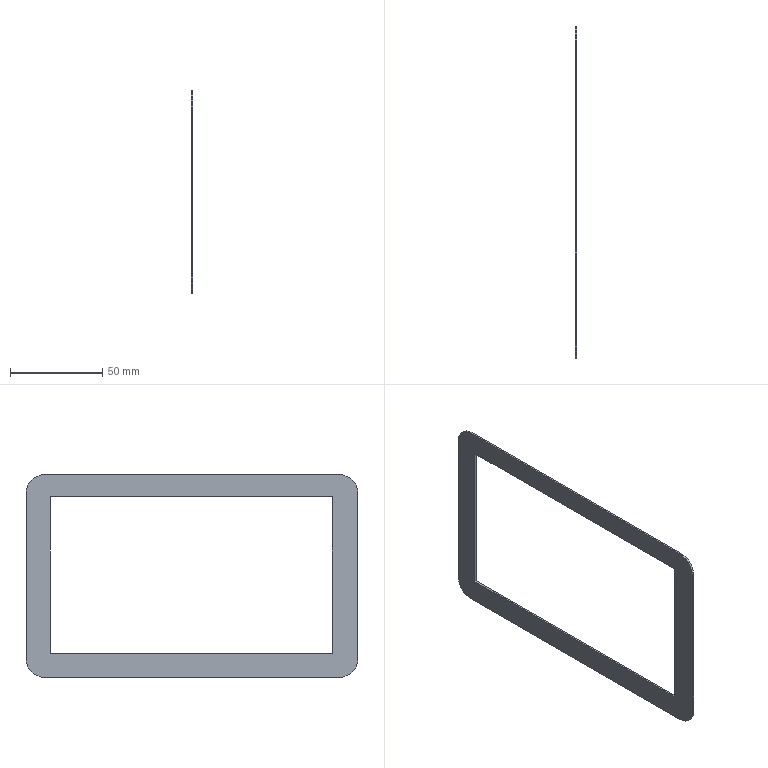Part | STEP file | RJ-HMS7-01_X2_58F34F5394A391D_4 | 1 solid | 14 faces | box 1 x 180 x 110 mm | volume 6715 mm3 | plane 10 | cylinder 4 | commonest cylinder face diameters 20 x4
STEP:
#1=CARTESIAN_POINT('',(0.,0.,0.));
#2=DIRECTION('',(0.,0.,1.));
#3=DIRECTION('',(1.,0.,0.));
#4=AXIS2_PLACEMENT_3D('',#1,#2,#3);
#5=CARTESIAN_POINT('',(770.3,4242.2,1279.394));
#6=VERTEX_POINT('',#5);
#7=CARTESIAN_POINT('',(770.3,4082.2,1279.394));
#8=VERTEX_POINT('',#7);
#9=CARTESIAN_POINT('',(770.3,4242.2,1279.394));
#10=DIRECTION('',(0.,-1.,0.));
#11=VECTOR('',#10,1.);
#12=LINE('',#9,#11);
#13=CARTESIAN_POINT('',(770.3,0.,0.));
#14=DIRECTION('',(1.,0.,0.));
#15=DIRECTION('',(0.,0.,-1.));
#16=AXIS2_PLACEMENT_3D('',#13,#14,#15);
#17=PLANE('',#16);
#18=CARTESIAN_POINT('',(-1279.394,4242.2));
#19=DIRECTION('',(0.,-1.));
#20=VECTOR('',#19,1.);
#21=LINE('',#18,#20);
#22=(GEOMETRIC_REPRESENTATION_CONTEXT(2)PARAMETRIC_REPRESENTATION_CONTEXT()REPRESENTATION_CONTEXT('',''));
#23=DEFINITIONAL_REPRESENTATION('',(#21),#22);
#24=PCURVE('',#17,#23);
#25=CARTESIAN_POINT('',(757.1,4072.2,1279.394));
#26=DIRECTION('',(0.,0.,-1.));
#27=DIRECTION('',(-1.,0.,0.));
#28=AXIS2_PLACEMENT_3D('',#25,#26,#27);
#29=PLANE('',#28);
#30=CARTESIAN_POINT('',(-13.2,170.));
#31=DIRECTION('',(0.,-1.));
#32=VECTOR('',#31,1.);
#33=LINE('',#30,#32);
#34=(GEOMETRIC_REPRESENTATION_CONTEXT(2)PARAMETRIC_REPRESENTATION_CONTEXT()REPRESENTATION_CONTEXT('',''));
#35=DEFINITIONAL_REPRESENTATION('',(#33),#34);
#36=PCURVE('',#29,#35);
#37=SURFACE_CURVE('',#12,(#24,#36),.PCURVE_S1.);
#38=EDGE_CURVE('',#6,#8,#37,.T.);
#39=ORIENTED_EDGE('',*,*,#38,.T.);
#40=CARTESIAN_POINT('',(770.3,4072.2,1289.394));
#41=VERTEX_POINT('',#40);
#42=CARTESIAN_POINT('',(770.3,4082.2,1289.394));
#43=DIRECTION('',(1.,0.,0.));
#44=DIRECTION('',(0.,-1.,0.));
#45=AXIS2_PLACEMENT_3D('',#42,#43,#44);
#46=CIRCLE('',#45,10.);
#47=CARTESIAN_POINT('',(-1289.394,4082.2));
#48=DIRECTION('',(0.,-1.));
#49=AXIS2_PLACEMENT_2D('',#47,#48);
#50=CIRCLE('',#49,10.);
#51=(GEOMETRIC_REPRESENTATION_CONTEXT(2)PARAMETRIC_REPRESENTATION_CONTEXT()REPRESENTATION_CONTEXT('',''));
#52=DEFINITIONAL_REPRESENTATION('',(#50),#51);
#53=PCURVE('',#17,#52);
#54=CARTESIAN_POINT('',(757.1,4082.2,1289.394));
#55=DIRECTION('',(-1.,0.,0.));
#56=DIRECTION('',(0.,0.,1.));
#57=AXIS2_PLACEMENT_3D('',#54,#55,#56);
#58=CYLINDRICAL_SURFACE('',#57,10.);
#59=CARTESIAN_POINT('',(4.712,-13.2));
#60=DIRECTION('',(-1.,0.));
#61=VECTOR('',#60,1.);
#62=LINE('',#59,#61);
#63=(GEOMETRIC_REPRESENTATION_CONTEXT(2)PARAMETRIC_REPRESENTATION_CONTEXT()REPRESENTATION_CONTEXT('',''));
#64=DEFINITIONAL_REPRESENTATION('',(#62),#63);
#65=PCURVE('',#58,#64);
#66=SURFACE_CURVE('',#46,(#53,#65),.PCURVE_S1.);
#67=EDGE_CURVE('',#41,#8,#66,.T.);
#68=ORIENTED_EDGE('',*,*,#67,.F.);
#69=CARTESIAN_POINT('',(770.3,4072.2,1379.394));
#70=VERTEX_POINT('',#69);
#71=CARTESIAN_POINT('',(770.3,4072.2,1289.394));
#72=DIRECTION('',(0.,0.,1.));
#73=VECTOR('',#72,1.);
#74=LINE('',#71,#73);
#75=CARTESIAN_POINT('',(-1289.394,4072.2));
#76=DIRECTION('',(-1.,0.));
#77=VECTOR('',#76,1.);
#78=LINE('',#75,#77);
#79=(GEOMETRIC_REPRESENTATION_CONTEXT(2)PARAMETRIC_REPRESENTATION_CONTEXT()REPRESENTATION_CONTEXT('',''));
#80=DEFINITIONAL_REPRESENTATION('',(#78),#79);
#81=PCURVE('',#17,#80);
#82=CARTESIAN_POINT('',(757.1,4072.2,1389.394));
#83=DIRECTION('',(0.,-1.,0.));
#84=DIRECTION('',(0.,0.,-1.));
#85=AXIS2_PLACEMENT_3D('',#82,#83,#84);
#86=PLANE('',#85);
#87=CARTESIAN_POINT('',(100.,13.2));
#88=DIRECTION('',(-1.,0.));
#89=VECTOR('',#88,1.);
#90=LINE('',#87,#89);
#91=(GEOMETRIC_REPRESENTATION_CONTEXT(2)PARAMETRIC_REPRESENTATION_CONTEXT()REPRESENTATION_CONTEXT('',''));
#92=DEFINITIONAL_REPRESENTATION('',(#90),#91);
#93=PCURVE('',#86,#92);
#94=SURFACE_CURVE('',#74,(#81,#93),.PCURVE_S1.);
#95=EDGE_CURVE('',#41,#70,#94,.T.);
#96=ORIENTED_EDGE('',*,*,#95,.T.);
#97=CARTESIAN_POINT('',(770.3,4082.2,1389.394));
#98=VERTEX_POINT('',#97);
#99=CARTESIAN_POINT('',(770.3,4082.2,1379.394));
#100=DIRECTION('',(1.,0.,0.));
#101=DIRECTION('',(0.,0.,1.));
#102=AXIS2_PLACEMENT_3D('',#99,#100,#101);
#103=CIRCLE('',#102,10.);
#104=CARTESIAN_POINT('',(-1379.394,4082.2));
#105=DIRECTION('',(-1.,0.));
#106=AXIS2_PLACEMENT_2D('',#104,#105);
#107=CIRCLE('',#106,10.);
#108=(GEOMETRIC_REPRESENTATION_CONTEXT(2)PARAMETRIC_REPRESENTATION_CONTEXT()REPRESENTATION_CONTEXT('',''));
#109=DEFINITIONAL_REPRESENTATION('',(#107),#108);
#110=PCURVE('',#17,#109);
#111=CARTESIAN_POINT('',(757.1,4082.2,1379.394));
#112=DIRECTION('',(-1.,0.,0.));
#113=DIRECTION('',(0.,0.,1.));
#114=AXIS2_PLACEMENT_3D('',#111,#112,#113);
#115=CYLINDRICAL_SURFACE('',#114,10.);
#116=CARTESIAN_POINT('',(6.283,-13.2));
#117=DIRECTION('',(-1.,0.));
#118=VECTOR('',#117,1.);
#119=LINE('',#116,#118);
#120=(GEOMETRIC_REPRESENTATION_CONTEXT(2)PARAMETRIC_REPRESENTATION_CONTEXT()REPRESENTATION_CONTEXT('',''));
#121=DEFINITIONAL_REPRESENTATION('',(#119),#120);
#122=PCURVE('',#115,#121);
#123=SURFACE_CURVE('',#103,(#110,#122),.PCURVE_S1.);
#124=EDGE_CURVE('',#98,#70,#123,.T.);
#125=ORIENTED_EDGE('',*,*,#124,.F.);
#126=CARTESIAN_POINT('',(770.3,4242.2,1389.394));
#127=VERTEX_POINT('',#126);
#128=CARTESIAN_POINT('',(770.3,4082.2,1389.394));
#129=DIRECTION('',(0.,1.,0.));
#130=VECTOR('',#129,1.);
#131=LINE('',#128,#130);
#132=CARTESIAN_POINT('',(-1389.394,4082.2));
#133=DIRECTION('',(0.,1.));
#134=VECTOR('',#133,1.);
#135=LINE('',#132,#134);
#136=(GEOMETRIC_REPRESENTATION_CONTEXT(2)PARAMETRIC_REPRESENTATION_CONTEXT()REPRESENTATION_CONTEXT('',''));
#137=DEFINITIONAL_REPRESENTATION('',(#135),#136);
#138=PCURVE('',#17,#137);
#139=CARTESIAN_POINT('',(757.1,4252.2,1389.394));
#140=DIRECTION('',(0.,0.,1.));
#141=DIRECTION('',(1.,0.,0.));
#142=AXIS2_PLACEMENT_3D('',#139,#140,#141);
#143=PLANE('',#142);
#144=CARTESIAN_POINT('',(13.2,-170.));
#145=DIRECTION('',(0.,1.));
#146=VECTOR('',#145,1.);
#147=LINE('',#144,#146);
#148=(GEOMETRIC_REPRESENTATION_CONTEXT(2)PARAMETRIC_REPRESENTATION_CONTEXT()REPRESENTATION_CONTEXT('',''));
#149=DEFINITIONAL_REPRESENTATION('',(#147),#148);
#150=PCURVE('',#143,#149);
#151=SURFACE_CURVE('',#131,(#138,#150),.PCURVE_S1.);
#152=EDGE_CURVE('',#98,#127,#151,.T.);
#153=ORIENTED_EDGE('',*,*,#152,.T.);
#154=CARTESIAN_POINT('',(770.3,4252.2,1379.394));
#155=VERTEX_POINT('',#154);
#156=CARTESIAN_POINT('',(770.3,4242.2,1379.394));
#157=DIRECTION('',(1.,0.,0.));
#158=DIRECTION('',(0.,1.,0.));
#159=AXIS2_PLACEMENT_3D('',#156,#157,#158);
#160=CIRCLE('',#159,10.);
#161=CARTESIAN_POINT('',(-1379.394,4242.2));
#162=DIRECTION('',(0.,1.));
#163=AXIS2_PLACEMENT_2D('',#161,#162);
#164=CIRCLE('',#163,10.);
#165=(GEOMETRIC_REPRESENTATION_CONTEXT(2)PARAMETRIC_REPRESENTATION_CONTEXT()REPRESENTATION_CONTEXT('',''));
#166=DEFINITIONAL_REPRESENTATION('',(#164),#165);
#167=PCURVE('',#17,#166);
#168=CARTESIAN_POINT('',(757.1,4242.2,1379.394));
#169=DIRECTION('',(-1.,0.,0.));
#170=DIRECTION('',(0.,0.,1.));
#171=AXIS2_PLACEMENT_3D('',#168,#169,#170);
#172=CYLINDRICAL_SURFACE('',#171,10.);
#173=CARTESIAN_POINT('',(1.571,-13.2));
#174=DIRECTION('',(-1.,0.));
#175=VECTOR('',#174,1.);
#176=LINE('',#173,#175);
#177=(GEOMETRIC_REPRESENTATION_CONTEXT(2)PARAMETRIC_REPRESENTATION_CONTEXT()REPRESENTATION_CONTEXT('',''));
#178=DEFINITIONAL_REPRESENTATION('',(#176),#177);
#179=PCURVE('',#172,#178);
#180=SURFACE_CURVE('',#160,(#167,#179),.PCURVE_S1.);
#181=EDGE_CURVE('',#155,#127,#180,.T.);
#182=ORIENTED_EDGE('',*,*,#181,.F.);
#183=CARTESIAN_POINT('',(770.3,4252.2,1289.394));
#184=VERTEX_POINT('',#183);
#185=CARTESIAN_POINT('',(770.3,4252.2,1379.394));
#186=DIRECTION('',(0.,0.,-1.));
#187=VECTOR('',#186,1.);
#188=LINE('',#185,#187);
#189=CARTESIAN_POINT('',(-1379.394,4252.2));
#190=DIRECTION('',(1.,0.));
#191=VECTOR('',#190,1.);
#192=LINE('',#189,#191);
#193=(GEOMETRIC_REPRESENTATION_CONTEXT(2)PARAMETRIC_REPRESENTATION_CONTEXT()REPRESENTATION_CONTEXT('',''));
#194=DEFINITIONAL_REPRESENTATION('',(#192),#193);
#195=PCURVE('',#17,#194);
#196=CARTESIAN_POINT('',(757.1,4252.2,1279.394));
#197=DIRECTION('',(0.,1.,0.));
#198=DIRECTION('',(0.,0.,1.));
#199=AXIS2_PLACEMENT_3D('',#196,#197,#198);
#200=PLANE('',#199);
#201=CARTESIAN_POINT('',(100.,13.2));
#202=DIRECTION('',(-1.,0.));
#203=VECTOR('',#202,1.);
#204=LINE('',#201,#203);
#205=(GEOMETRIC_REPRESENTATION_CONTEXT(2)PARAMETRIC_REPRESENTATION_CONTEXT()REPRESENTATION_CONTEXT('',''));
#206=DEFINITIONAL_REPRESENTATION('',(#204),#205);
#207=PCURVE('',#200,#206);
#208=SURFACE_CURVE('',#188,(#195,#207),.PCURVE_S1.);
#209=EDGE_CURVE('',#155,#184,#208,.T.);
#210=ORIENTED_EDGE('',*,*,#209,.T.);
#211=CARTESIAN_POINT('',(770.3,4242.2,1289.394));
#212=DIRECTION('',(1.,0.,0.));
#213=DIRECTION('',(0.,0.,-1.));
#214=AXIS2_PLACEMENT_3D('',#211,#212,#213);
#215=CIRCLE('',#214,10.);
#216=CARTESIAN_POINT('',(-1289.394,4242.2));
#217=DIRECTION('',(1.,0.));
#218=AXIS2_PLACEMENT_2D('',#216,#217);
#219=CIRCLE('',#218,10.);
#220=(GEOMETRIC_REPRESENTATION_CONTEXT(2)PARAMETRIC_REPRESENTATION_CONTEXT()REPRESENTATION_CONTEXT('',''));
#221=DEFINITIONAL_REPRESENTATION('',(#219),#220);
#222=PCURVE('',#17,#221);
#223=CARTESIAN_POINT('',(757.1,4242.2,1289.394));
#224=DIRECTION('',(-1.,0.,0.));
#225=DIRECTION('',(0.,0.,1.));
#226=AXIS2_PLACEMENT_3D('',#223,#224,#225);
#227=CYLINDRICAL_SURFACE('',#226,10.);
#228=CARTESIAN_POINT('',(3.142,-13.2));
#229=DIRECTION('',(-1.,0.));
#230=VECTOR('',#229,1.);
#231=LINE('',#228,#230);
#232=(GEOMETRIC_REPRESENTATION_CONTEXT(2)PARAMETRIC_REPRESENTATION_CONTEXT()REPRESENTATION_CONTEXT('',''));
#233=DEFINITIONAL_REPRESENTATION('',(#231),#232);
#234=PCURVE('',#227,#233);
#235=SURFACE_CURVE('',#215,(#222,#234),.PCURVE_S1.);
#236=EDGE_CURVE('',#6,#184,#235,.T.);
#237=ORIENTED_EDGE('',*,*,#236,.F.);
#238=EDGE_LOOP('',(#39,#68,#96,#125,#153,#182,#210,#237));
#239=FACE_BOUND('',#238,.F.);
#240=CARTESIAN_POINT('',(770.3,4086.16,1377.354));
#241=VERTEX_POINT('',#240);
#242=CARTESIAN_POINT('',(770.3,4086.16,1292.434));
#243=VERTEX_POINT('',#242);
#244=CARTESIAN_POINT('',(770.3,4086.16,1377.354));
#245=DIRECTION('',(0.,0.,-1.));
#246=VECTOR('',#245,1.);
#247=LINE('',#244,#246);
#248=CARTESIAN_POINT('',(-1377.354,4086.16));
#249=DIRECTION('',(1.,0.));
#250=VECTOR('',#249,1.);
#251=LINE('',#248,#250);
#252=(GEOMETRIC_REPRESENTATION_CONTEXT(2)PARAMETRIC_REPRESENTATION_CONTEXT()REPRESENTATION_CONTEXT('',''));
#253=DEFINITIONAL_REPRESENTATION('',(#251),#252);
#254=PCURVE('',#17,#253);
#255=CARTESIAN_POINT('',(770.3,4086.16,1291.434));
#256=DIRECTION('',(0.,-1.,0.));
#257=DIRECTION('',(0.,0.,-1.));
#258=AXIS2_PLACEMENT_3D('',#255,#256,#257);
#259=PLANE('',#258);
#260=CARTESIAN_POINT('',(-85.92,0.));
#261=DIRECTION('',(1.,0.));
#262=VECTOR('',#261,1.);
#263=LINE('',#260,#262);
#264=(GEOMETRIC_REPRESENTATION_CONTEXT(2)PARAMETRIC_REPRESENTATION_CONTEXT()REPRESENTATION_CONTEXT('',''));
#265=DEFINITIONAL_REPRESENTATION('',(#263),#264);
#266=PCURVE('',#259,#265);
#267=SURFACE_CURVE('',#247,(#254,#266),.PCURVE_S1.);
#268=EDGE_CURVE('',#241,#243,#267,.T.);
#269=ORIENTED_EDGE('',*,*,#268,.T.);
#270=CARTESIAN_POINT('',(770.3,4239.24,1292.434));
#271=VERTEX_POINT('',#270);
#272=CARTESIAN_POINT('',(770.3,4086.16,1292.434));
#273=DIRECTION('',(0.,1.,0.));
#274=VECTOR('',#273,1.);
#275=LINE('',#272,#274);
#276=CARTESIAN_POINT('',(-1292.434,4086.16));
#277=DIRECTION('',(0.,1.));
#278=VECTOR('',#277,1.);
#279=LINE('',#276,#278);
#280=(GEOMETRIC_REPRESENTATION_CONTEXT(2)PARAMETRIC_REPRESENTATION_CONTEXT()REPRESENTATION_CONTEXT('',''));
#281=DEFINITIONAL_REPRESENTATION('',(#279),#280);
#282=PCURVE('',#17,#281);
#283=CARTESIAN_POINT('',(770.3,4239.24,1292.434));
#284=DIRECTION('',(0.,0.,-1.));
#285=DIRECTION('',(-1.,0.,0.));
#286=AXIS2_PLACEMENT_3D('',#283,#284,#285);
#287=PLANE('',#286);
#288=CARTESIAN_POINT('',(0.,-153.08));
#289=DIRECTION('',(0.,1.));
#290=VECTOR('',#289,1.);
#291=LINE('',#288,#290);
#292=(GEOMETRIC_REPRESENTATION_CONTEXT(2)PARAMETRIC_REPRESENTATION_CONTEXT()REPRESENTATION_CONTEXT('',''));
#293=DEFINITIONAL_REPRESENTATION('',(#291),#292);
#294=PCURVE('',#287,#293);
#295=SURFACE_CURVE('',#275,(#282,#294),.PCURVE_S1.);
#296=EDGE_CURVE('',#243,#271,#295,.T.);
#297=ORIENTED_EDGE('',*,*,#296,.T.);
#298=CARTESIAN_POINT('',(770.3,4239.24,1377.354));
#299=VERTEX_POINT('',#298);
#300=CARTESIAN_POINT('',(770.3,4239.24,1292.434));
#301=DIRECTION('',(0.,0.,1.));
#302=VECTOR('',#301,1.);
#303=LINE('',#300,#302);
#304=CARTESIAN_POINT('',(-1292.434,4239.24));
#305=DIRECTION('',(-1.,0.));
#306=VECTOR('',#305,1.);
#307=LINE('',#304,#306);
#308=(GEOMETRIC_REPRESENTATION_CONTEXT(2)PARAMETRIC_REPRESENTATION_CONTEXT()REPRESENTATION_CONTEXT('',''));
#309=DEFINITIONAL_REPRESENTATION('',(#307),#308);
#310=PCURVE('',#17,#309);
#311=CARTESIAN_POINT('',(770.3,4239.24,1377.354));
#312=DIRECTION('',(0.,1.,0.));
#313=DIRECTION('',(0.,0.,1.));
#314=AXIS2_PLACEMENT_3D('',#311,#312,#313);
#315=PLANE('',#314);
#316=CARTESIAN_POINT('',(-84.92,0.));
#317=DIRECTION('',(1.,0.));
#318=VECTOR('',#317,1.);
#319=LINE('',#316,#318);
#320=(GEOMETRIC_REPRESENTATION_CONTEXT(2)PARAMETRIC_REPRESENTATION_CONTEXT()REPRESENTATION_CONTEXT('',''));
#321=DEFINITIONAL_REPRESENTATION('',(#319),#320);
#322=PCURVE('',#315,#321);
#323=SURFACE_CURVE('',#303,(#310,#322),.PCURVE_S1.);
#324=EDGE_CURVE('',#271,#299,#323,.T.);
#325=ORIENTED_EDGE('',*,*,#324,.T.);
#326=CARTESIAN_POINT('',(770.3,4239.24,1377.354));
#327=DIRECTION('',(0.,-1.,0.));
#328=VECTOR('',#327,1.);
#329=LINE('',#326,#328);
#330=CARTESIAN_POINT('',(-1377.354,4239.24));
#331=DIRECTION('',(0.,-1.));
#332=VECTOR('',#331,1.);
#333=LINE('',#330,#332);
#334=(GEOMETRIC_REPRESENTATION_CONTEXT(2)PARAMETRIC_REPRESENTATION_CONTEXT()REPRESENTATION_CONTEXT('',''));
#335=DEFINITIONAL_REPRESENTATION('',(#333),#334);
#336=PCURVE('',#17,#335);
#337=CARTESIAN_POINT('',(770.3,4085.16,1377.354));
#338=DIRECTION('',(0.,0.,1.));
#339=DIRECTION('',(1.,0.,0.));
#340=AXIS2_PLACEMENT_3D('',#337,#338,#339);
#341=PLANE('',#340);
#342=CARTESIAN_POINT('',(0.,154.08));
#343=DIRECTION('',(0.,-1.));
#344=VECTOR('',#343,1.);
#345=LINE('',#342,#344);
#346=(GEOMETRIC_REPRESENTATION_CONTEXT(2)PARAMETRIC_REPRESENTATION_CONTEXT()REPRESENTATION_CONTEXT('',''));
#347=DEFINITIONAL_REPRESENTATION('',(#345),#346);
#348=PCURVE('',#341,#347);
#349=SURFACE_CURVE('',#329,(#336,#348),.PCURVE_S1.);
#350=EDGE_CURVE('',#299,#241,#349,.T.);
#351=ORIENTED_EDGE('',*,*,#350,.T.);
#352=EDGE_LOOP('',(#269,#297,#325,#351));
#353=FACE_BOUND('',#352,.F.);
#354=ADVANCED_FACE('',(#239,#353),#17,.T.);
#355=CARTESIAN_POINT('',(769.3,4086.16,1377.354));
#356=VERTEX_POINT('',#355);
#357=CARTESIAN_POINT('',(769.3,4086.16,1292.434));
#358=VERTEX_POINT('',#357);
#359=CARTESIAN_POINT('',(769.3,4086.16,1377.354));
#360=DIRECTION('',(0.,0.,-1.));
#361=VECTOR('',#360,1.);
#362=LINE('',#359,#361);
#363=CARTESIAN_POINT('',(-85.92,-1.));
#364=DIRECTION('',(1.,0.));
#365=VECTOR('',#364,1.);
#366=LINE('',#363,#365);
#367=(GEOMETRIC_REPRESENTATION_CONTEXT(2)PARAMETRIC_REPRESENTATION_CONTEXT()REPRESENTATION_CONTEXT('',''));
#368=DEFINITIONAL_REPRESENTATION('',(#366),#367);
#369=PCURVE('',#259,#368);
#370=CARTESIAN_POINT('',(769.3,0.,0.));
#371=DIRECTION('',(1.,0.,0.));
#372=DIRECTION('',(0.,0.,-1.));
#373=AXIS2_PLACEMENT_3D('',#370,#371,#372);
#374=PLANE('',#373);
#375=CARTESIAN_POINT('',(-1377.354,4086.16));
#376=DIRECTION('',(1.,0.));
#377=VECTOR('',#376,1.);
#378=LINE('',#375,#377);
#379=(GEOMETRIC_REPRESENTATION_CONTEXT(2)PARAMETRIC_REPRESENTATION_CONTEXT()REPRESENTATION_CONTEXT('',''));
#380=DEFINITIONAL_REPRESENTATION('',(#378),#379);
#381=PCURVE('',#374,#380);
#382=SURFACE_CURVE('',#362,(#369,#381),.PCURVE_S1.);
#383=EDGE_CURVE('',#356,#358,#382,.T.);
#384=ORIENTED_EDGE('',*,*,#383,.T.);
#385=CARTESIAN_POINT('',(769.3,4086.16,1292.434));
#386=DIRECTION('',(1.,0.,0.));
#387=VECTOR('',#386,1.);
#388=LINE('',#385,#387);
#389=CARTESIAN_POINT('',(-1.,-1.));
#390=DIRECTION('',(0.,1.));
#391=VECTOR('',#390,1.);
#392=LINE('',#389,#391);
#393=(GEOMETRIC_REPRESENTATION_CONTEXT(2)PARAMETRIC_REPRESENTATION_CONTEXT()REPRESENTATION_CONTEXT('',''));
#394=DEFINITIONAL_REPRESENTATION('',(#392),#393);
#395=PCURVE('',#259,#394);
#396=CARTESIAN_POINT('',(1.,-153.08));
#397=DIRECTION('',(-1.,0.));
#398=VECTOR('',#397,1.);
#399=LINE('',#396,#398);
#400=(GEOMETRIC_REPRESENTATION_CONTEXT(2)PARAMETRIC_REPRESENTATION_CONTEXT()REPRESENTATION_CONTEXT('',''));
#401=DEFINITIONAL_REPRESENTATION('',(#399),#400);
#402=PCURVE('',#287,#401);
#403=SURFACE_CURVE('',#388,(#395,#402),.PCURVE_S1.);
#404=EDGE_CURVE('',#358,#243,#403,.T.);
#405=ORIENTED_EDGE('',*,*,#404,.T.);
#406=ORIENTED_EDGE('',*,*,#268,.F.);
#407=CARTESIAN_POINT('',(769.3,4086.16,1377.354));
#408=DIRECTION('',(1.,0.,0.));
#409=VECTOR('',#408,1.);
#410=LINE('',#407,#409);
#411=CARTESIAN_POINT('',(-85.92,-1.));
#412=DIRECTION('',(0.,1.));
#413=VECTOR('',#412,1.);
#414=LINE('',#411,#413);
#415=(GEOMETRIC_REPRESENTATION_CONTEXT(2)PARAMETRIC_REPRESENTATION_CONTEXT()REPRESENTATION_CONTEXT('',''));
#416=DEFINITIONAL_REPRESENTATION('',(#414),#415);
#417=PCURVE('',#259,#416);
#418=CARTESIAN_POINT('',(-1.,1.));
#419=DIRECTION('',(1.,0.));
#420=VECTOR('',#419,1.);
#421=LINE('',#418,#420);
#422=(GEOMETRIC_REPRESENTATION_CONTEXT(2)PARAMETRIC_REPRESENTATION_CONTEXT()REPRESENTATION_CONTEXT('',''));
#423=DEFINITIONAL_REPRESENTATION('',(#421),#422);
#424=PCURVE('',#341,#423);
#425=SURFACE_CURVE('',#410,(#417,#424),.PCURVE_S1.);
#426=EDGE_CURVE('',#356,#241,#425,.T.);
#427=ORIENTED_EDGE('',*,*,#426,.F.);
#428=EDGE_LOOP('',(#384,#405,#406,#427));
#429=FACE_BOUND('',#428,.F.);
#430=ADVANCED_FACE('',(#429),#259,.F.);
#431=CARTESIAN_POINT('',(769.3,4252.2,1379.394));
#432=VERTEX_POINT('',#431);
#433=CARTESIAN_POINT('',(769.3,4252.2,1289.394));
#434=VERTEX_POINT('',#433);
#435=CARTESIAN_POINT('',(769.3,4252.2,1379.394));
#436=DIRECTION('',(0.,0.,-1.));
#437=VECTOR('',#436,1.);
#438=LINE('',#435,#437);
#439=CARTESIAN_POINT('',(-1379.394,4252.2));
#440=DIRECTION('',(1.,0.));
#441=VECTOR('',#440,1.);
#442=LINE('',#439,#441);
#443=(GEOMETRIC_REPRESENTATION_CONTEXT(2)PARAMETRIC_REPRESENTATION_CONTEXT()REPRESENTATION_CONTEXT('',''));
#444=DEFINITIONAL_REPRESENTATION('',(#442),#443);
#445=PCURVE('',#374,#444);
#446=CARTESIAN_POINT('',(100.,12.2));
#447=DIRECTION('',(-1.,0.));
#448=VECTOR('',#447,1.);
#449=LINE('',#446,#448);
#450=(GEOMETRIC_REPRESENTATION_CONTEXT(2)PARAMETRIC_REPRESENTATION_CONTEXT()REPRESENTATION_CONTEXT('',''));
#451=DEFINITIONAL_REPRESENTATION('',(#449),#450);
#452=PCURVE('',#200,#451);
#453=SURFACE_CURVE('',#438,(#445,#452),.PCURVE_S1.);
#454=EDGE_CURVE('',#432,#434,#453,.T.);
#455=ORIENTED_EDGE('',*,*,#454,.F.);
#456=CARTESIAN_POINT('',(769.3,4242.2,1389.394));
#457=VERTEX_POINT('',#456);
#458=CARTESIAN_POINT('',(769.3,4242.2,1379.394));
#459=DIRECTION('',(-1.,0.,0.));
#460=DIRECTION('',(0.,0.,1.));
#461=AXIS2_PLACEMENT_3D('',#458,#459,#460);
#462=CIRCLE('',#461,10.);
#463=CARTESIAN_POINT('',(-1389.394,4242.2));
#464=CARTESIAN_POINT('',(-1389.394,4259.521));
#465=CARTESIAN_POINT('',(-1374.394,4250.86));
#466=CARTESIAN_POINT('',(-1359.394,4242.2));
#467=CARTESIAN_POINT('',(-1374.394,4233.54));
#468=CARTESIAN_POINT('',(-1389.394,4224.879));
#469=CARTESIAN_POINT('',(-1389.394,4242.2));
#470=(BOUNDED_CURVE()B_SPLINE_CURVE(2,(#463,#464,#465,#466,#467,#468,#469),.UNSPECIFIED.,.T.,.F.)B_SPLINE_CURVE_WITH_KNOTS((1,2,2,2,2,1),(-2.094,0.,2.094,4.189,6.283,8.378),.UNSPECIFIED.)CURVE()GEOMETRIC_REPRESENTATION_ITEM()RATIONAL_B_SPLINE_CURVE((1.,0.5,1.,0.5,1.,0.5,1.))REPRESENTATION_ITEM(''));
#471=(GEOMETRIC_REPRESENTATION_CONTEXT(2)PARAMETRIC_REPRESENTATION_CONTEXT()REPRESENTATION_CONTEXT('',''));
#472=DEFINITIONAL_REPRESENTATION('',(#470),#471);
#473=PCURVE('',#374,#472);
#474=CARTESIAN_POINT('',(0.,-12.2));
#475=DIRECTION('',(1.,0.));
#476=VECTOR('',#475,1.);
#477=LINE('',#474,#476);
#478=(GEOMETRIC_REPRESENTATION_CONTEXT(2)PARAMETRIC_REPRESENTATION_CONTEXT()REPRESENTATION_CONTEXT('',''));
#479=DEFINITIONAL_REPRESENTATION('',(#477),#478);
#480=PCURVE('',#172,#479);
#481=SURFACE_CURVE('',#462,(#473,#480),.PCURVE_S1.);
#482=EDGE_CURVE('',#457,#432,#481,.T.);
#483=ORIENTED_EDGE('',*,*,#482,.F.);
#484=CARTESIAN_POINT('',(769.3,4082.2,1389.394));
#485=VERTEX_POINT('',#484);
#486=CARTESIAN_POINT('',(769.3,4082.2,1389.394));
#487=DIRECTION('',(0.,1.,0.));
#488=VECTOR('',#487,1.);
#489=LINE('',#486,#488);
#490=CARTESIAN_POINT('',(-1389.394,4082.2));
#491=DIRECTION('',(0.,1.));
#492=VECTOR('',#491,1.);
#493=LINE('',#490,#492);
#494=(GEOMETRIC_REPRESENTATION_CONTEXT(2)PARAMETRIC_REPRESENTATION_CONTEXT()REPRESENTATION_CONTEXT('',''));
#495=DEFINITIONAL_REPRESENTATION('',(#493),#494);
#496=PCURVE('',#374,#495);
#497=CARTESIAN_POINT('',(12.2,-170.));
#498=DIRECTION('',(0.,1.));
#499=VECTOR('',#498,1.);
#500=LINE('',#497,#499);
#501=(GEOMETRIC_REPRESENTATION_CONTEXT(2)PARAMETRIC_REPRESENTATION_CONTEXT()REPRESENTATION_CONTEXT('',''));
#502=DEFINITIONAL_REPRESENTATION('',(#500),#501);
#503=PCURVE('',#143,#502);
#504=SURFACE_CURVE('',#489,(#496,#503),.PCURVE_S1.);
#505=EDGE_CURVE('',#485,#457,#504,.T.);
#506=ORIENTED_EDGE('',*,*,#505,.F.);
#507=CARTESIAN_POINT('',(769.3,4072.2,1379.394));
#508=VERTEX_POINT('',#507);
#509=CARTESIAN_POINT('',(769.3,4082.2,1379.394));
#510=DIRECTION('',(-1.,0.,0.));
#511=DIRECTION('',(0.,-1.,0.));
#512=AXIS2_PLACEMENT_3D('',#509,#510,#511);
#513=CIRCLE('',#512,10.);
#514=CARTESIAN_POINT('',(-1379.394,4072.2));
#515=CARTESIAN_POINT('',(-1396.714,4072.2));
#516=CARTESIAN_POINT('',(-1388.054,4087.2));
#517=CARTESIAN_POINT('',(-1379.394,4102.2));
#518=CARTESIAN_POINT('',(-1370.733,4087.2));
#519=CARTESIAN_POINT('',(-1362.073,4072.2));
#520=CARTESIAN_POINT('',(-1379.394,4072.2));
#521=(BOUNDED_CURVE()B_SPLINE_CURVE(2,(#514,#515,#516,#517,#518,#519,#520),.UNSPECIFIED.,.T.,.F.)B_SPLINE_CURVE_WITH_KNOTS((1,2,2,2,2,1),(-2.094,0.,2.094,4.189,6.283,8.378),.UNSPECIFIED.)CURVE()GEOMETRIC_REPRESENTATION_ITEM()RATIONAL_B_SPLINE_CURVE((1.,0.5,1.,0.5,1.,0.5,1.))REPRESENTATION_ITEM(''));
#522=(GEOMETRIC_REPRESENTATION_CONTEXT(2)PARAMETRIC_REPRESENTATION_CONTEXT()REPRESENTATION_CONTEXT('',''));
#523=DEFINITIONAL_REPRESENTATION('',(#521),#522);
#524=PCURVE('',#374,#523);
#525=CARTESIAN_POINT('',(4.712,-12.2));
#526=DIRECTION('',(1.,0.));
#527=VECTOR('',#526,1.);
#528=LINE('',#525,#527);
#529=(GEOMETRIC_REPRESENTATION_CONTEXT(2)PARAMETRIC_REPRESENTATION_CONTEXT()REPRESENTATION_CONTEXT('',''));
#530=DEFINITIONAL_REPRESENTATION('',(#528),#529);
#531=PCURVE('',#115,#530);
#532=SURFACE_CURVE('',#513,(#524,#531),.PCURVE_S1.);
#533=EDGE_CURVE('',#508,#485,#532,.T.);
#534=ORIENTED_EDGE('',*,*,#533,.F.);
#535=CARTESIAN_POINT('',(769.3,4072.2,1289.394));
#536=VERTEX_POINT('',#535);
#537=CARTESIAN_POINT('',(769.3,4072.2,1289.394));
#538=DIRECTION('',(0.,0.,1.));
#539=VECTOR('',#538,1.);
#540=LINE('',#537,#539);
#541=CARTESIAN_POINT('',(-1289.394,4072.2));
#542=DIRECTION('',(-1.,0.));
#543=VECTOR('',#542,1.);
#544=LINE('',#541,#543);
#545=(GEOMETRIC_REPRESENTATION_CONTEXT(2)PARAMETRIC_REPRESENTATION_CONTEXT()REPRESENTATION_CONTEXT('',''));
#546=DEFINITIONAL_REPRESENTATION('',(#544),#545);
#547=PCURVE('',#374,#546);
#548=CARTESIAN_POINT('',(100.,12.2));
#549=DIRECTION('',(-1.,0.));
#550=VECTOR('',#549,1.);
#551=LINE('',#548,#550);
#552=(GEOMETRIC_REPRESENTATION_CONTEXT(2)PARAMETRIC_REPRESENTATION_CONTEXT()REPRESENTATION_CONTEXT('',''));
#553=DEFINITIONAL_REPRESENTATION('',(#551),#552);
#554=PCURVE('',#86,#553);
#555=SURFACE_CURVE('',#540,(#547,#554),.PCURVE_S1.);
#556=EDGE_CURVE('',#536,#508,#555,.T.);
#557=ORIENTED_EDGE('',*,*,#556,.F.);
#558=CARTESIAN_POINT('',(769.3,4082.2,1279.394));
#559=VERTEX_POINT('',#558);
#560=CARTESIAN_POINT('',(769.3,4082.2,1289.394));
#561=DIRECTION('',(-1.,0.,0.));
#562=DIRECTION('',(0.,0.,-1.));
#563=AXIS2_PLACEMENT_3D('',#560,#561,#562);
#564=CIRCLE('',#563,10.);
#565=CARTESIAN_POINT('',(-1279.394,4082.2));
#566=CARTESIAN_POINT('',(-1279.394,4064.879));
#567=CARTESIAN_POINT('',(-1294.394,4073.54));
#568=CARTESIAN_POINT('',(-1309.394,4082.2));
#569=CARTESIAN_POINT('',(-1294.394,4090.86));
#570=CARTESIAN_POINT('',(-1279.394,4099.521));
#571=CARTESIAN_POINT('',(-1279.394,4082.2));
#572=(BOUNDED_CURVE()B_SPLINE_CURVE(2,(#565,#566,#567,#568,#569,#570,#571),.UNSPECIFIED.,.T.,.F.)B_SPLINE_CURVE_WITH_KNOTS((1,2,2,2,2,1),(-2.094,0.,2.094,4.189,6.283,8.378),.UNSPECIFIED.)CURVE()GEOMETRIC_REPRESENTATION_ITEM()RATIONAL_B_SPLINE_CURVE((1.,0.5,1.,0.5,1.,0.5,1.))REPRESENTATION_ITEM(''));
#573=(GEOMETRIC_REPRESENTATION_CONTEXT(2)PARAMETRIC_REPRESENTATION_CONTEXT()REPRESENTATION_CONTEXT('',''));
#574=DEFINITIONAL_REPRESENTATION('',(#572),#573);
#575=PCURVE('',#374,#574);
#576=CARTESIAN_POINT('',(3.142,-12.2));
#577=DIRECTION('',(1.,0.));
#578=VECTOR('',#577,1.);
#579=LINE('',#576,#578);
#580=(GEOMETRIC_REPRESENTATION_CONTEXT(2)PARAMETRIC_REPRESENTATION_CONTEXT()REPRESENTATION_CONTEXT('',''));
#581=DEFINITIONAL_REPRESENTATION('',(#579),#580);
#582=PCURVE('',#58,#581);
#583=SURFACE_CURVE('',#564,(#575,#582),.PCURVE_S1.);
#584=EDGE_CURVE('',#559,#536,#583,.T.);
#585=ORIENTED_EDGE('',*,*,#584,.F.);
#586=CARTESIAN_POINT('',(769.3,4242.2,1279.394));
#587=VERTEX_POINT('',#586);
#588=CARTESIAN_POINT('',(769.3,4242.2,1279.394));
#589=DIRECTION('',(0.,-1.,0.));
#590=VECTOR('',#589,1.);
#591=LINE('',#588,#590);
#592=CARTESIAN_POINT('',(-1279.394,4242.2));
#593=DIRECTION('',(0.,-1.));
#594=VECTOR('',#593,1.);
#595=LINE('',#592,#594);
#596=(GEOMETRIC_REPRESENTATION_CONTEXT(2)PARAMETRIC_REPRESENTATION_CONTEXT()REPRESENTATION_CONTEXT('',''));
#597=DEFINITIONAL_REPRESENTATION('',(#595),#596);
#598=PCURVE('',#374,#597);
#599=CARTESIAN_POINT('',(-12.2,170.));
#600=DIRECTION('',(0.,-1.));
#601=VECTOR('',#600,1.);
#602=LINE('',#599,#601);
#603=(GEOMETRIC_REPRESENTATION_CONTEXT(2)PARAMETRIC_REPRESENTATION_CONTEXT()REPRESENTATION_CONTEXT('',''));
#604=DEFINITIONAL_REPRESENTATION('',(#602),#603);
#605=PCURVE('',#29,#604);
#606=SURFACE_CURVE('',#591,(#598,#605),.PCURVE_S1.);
#607=EDGE_CURVE('',#587,#559,#606,.T.);
#608=ORIENTED_EDGE('',*,*,#607,.F.);
#609=CARTESIAN_POINT('',(769.3,4242.2,1289.394));
#610=DIRECTION('',(-1.,0.,0.));
#611=DIRECTION('',(0.,1.,0.));
#612=AXIS2_PLACEMENT_3D('',#609,#610,#611);
#613=CIRCLE('',#612,10.);
#614=CARTESIAN_POINT('',(-1289.394,4252.2));
#615=CARTESIAN_POINT('',(-1272.073,4252.2));
#616=CARTESIAN_POINT('',(-1280.733,4237.2));
#617=CARTESIAN_POINT('',(-1289.394,4222.2));
#618=CARTESIAN_POINT('',(-1298.054,4237.2));
#619=CARTESIAN_POINT('',(-1306.714,4252.2));
#620=CARTESIAN_POINT('',(-1289.394,4252.2));
#621=(BOUNDED_CURVE()B_SPLINE_CURVE(2,(#614,#615,#616,#617,#618,#619,#620),.UNSPECIFIED.,.T.,.F.)B_SPLINE_CURVE_WITH_KNOTS((1,2,2,2,2,1),(-2.094,0.,2.094,4.189,6.283,8.378),.UNSPECIFIED.)CURVE()GEOMETRIC_REPRESENTATION_ITEM()RATIONAL_B_SPLINE_CURVE((1.,0.5,1.,0.5,1.,0.5,1.))REPRESENTATION_ITEM(''));
#622=(GEOMETRIC_REPRESENTATION_CONTEXT(2)PARAMETRIC_REPRESENTATION_CONTEXT()REPRESENTATION_CONTEXT('',''));
#623=DEFINITIONAL_REPRESENTATION('',(#621),#622);
#624=PCURVE('',#374,#623);
#625=CARTESIAN_POINT('',(1.571,-12.2));
#626=DIRECTION('',(1.,0.));
#627=VECTOR('',#626,1.);
#628=LINE('',#625,#627);
#629=(GEOMETRIC_REPRESENTATION_CONTEXT(2)PARAMETRIC_REPRESENTATION_CONTEXT()REPRESENTATION_CONTEXT('',''));
#630=DEFINITIONAL_REPRESENTATION('',(#628),#629);
#631=PCURVE('',#227,#630);
#632=SURFACE_CURVE('',#613,(#624,#631),.PCURVE_S1.);
#633=EDGE_CURVE('',#434,#587,#632,.T.);
#634=ORIENTED_EDGE('',*,*,#633,.F.);
#635=EDGE_LOOP('',(#455,#483,#506,#534,#557,#585,#608,#634));
#636=FACE_BOUND('',#635,.F.);
#637=ORIENTED_EDGE('',*,*,#383,.F.);
#638=CARTESIAN_POINT('',(769.3,4239.24,1377.354));
#639=VERTEX_POINT('',#638);
#640=CARTESIAN_POINT('',(769.3,4239.24,1377.354));
#641=DIRECTION('',(0.,-1.,0.));
#642=VECTOR('',#641,1.);
#643=LINE('',#640,#642);
#644=CARTESIAN_POINT('',(-1377.354,4239.24));
#645=DIRECTION('',(0.,-1.));
#646=VECTOR('',#645,1.);
#647=LINE('',#644,#646);
#648=(GEOMETRIC_REPRESENTATION_CONTEXT(2)PARAMETRIC_REPRESENTATION_CONTEXT()REPRESENTATION_CONTEXT('',''));
#649=DEFINITIONAL_REPRESENTATION('',(#647),#648);
#650=PCURVE('',#374,#649);
#651=CARTESIAN_POINT('',(-1.,154.08));
#652=DIRECTION('',(0.,-1.));
#653=VECTOR('',#652,1.);
#654=LINE('',#651,#653);
#655=(GEOMETRIC_REPRESENTATION_CONTEXT(2)PARAMETRIC_REPRESENTATION_CONTEXT()REPRESENTATION_CONTEXT('',''));
#656=DEFINITIONAL_REPRESENTATION('',(#654),#655);
#657=PCURVE('',#341,#656);
#658=SURFACE_CURVE('',#643,(#650,#657),.PCURVE_S1.);
#659=EDGE_CURVE('',#639,#356,#658,.T.);
#660=ORIENTED_EDGE('',*,*,#659,.F.);
#661=CARTESIAN_POINT('',(769.3,4239.24,1292.434));
#662=VERTEX_POINT('',#661);
#663=CARTESIAN_POINT('',(769.3,4239.24,1292.434));
#664=DIRECTION('',(0.,0.,1.));
#665=VECTOR('',#664,1.);
#666=LINE('',#663,#665);
#667=CARTESIAN_POINT('',(-1292.434,4239.24));
#668=DIRECTION('',(-1.,0.));
#669=VECTOR('',#668,1.);
#670=LINE('',#667,#669);
#671=(GEOMETRIC_REPRESENTATION_CONTEXT(2)PARAMETRIC_REPRESENTATION_CONTEXT()REPRESENTATION_CONTEXT('',''));
#672=DEFINITIONAL_REPRESENTATION('',(#670),#671);
#673=PCURVE('',#374,#672);
#674=CARTESIAN_POINT('',(-84.92,-1.));
#675=DIRECTION('',(1.,0.));
#676=VECTOR('',#675,1.);
#677=LINE('',#674,#676);
#678=(GEOMETRIC_REPRESENTATION_CONTEXT(2)PARAMETRIC_REPRESENTATION_CONTEXT()REPRESENTATION_CONTEXT('',''));
#679=DEFINITIONAL_REPRESENTATION('',(#677),#678);
#680=PCURVE('',#315,#679);
#681=SURFACE_CURVE('',#666,(#673,#680),.PCURVE_S1.);
#682=EDGE_CURVE('',#662,#639,#681,.T.);
#683=ORIENTED_EDGE('',*,*,#682,.F.);
#684=CARTESIAN_POINT('',(769.3,4086.16,1292.434));
#685=DIRECTION('',(0.,1.,0.));
#686=VECTOR('',#685,1.);
#687=LINE('',#684,#686);
#688=CARTESIAN_POINT('',(-1292.434,4086.16));
#689=DIRECTION('',(0.,1.));
#690=VECTOR('',#689,1.);
#691=LINE('',#688,#690);
#692=(GEOMETRIC_REPRESENTATION_CONTEXT(2)PARAMETRIC_REPRESENTATION_CONTEXT()REPRESENTATION_CONTEXT('',''));
#693=DEFINITIONAL_REPRESENTATION('',(#691),#692);
#694=PCURVE('',#374,#693);
#695=CARTESIAN_POINT('',(1.,-153.08));
#696=DIRECTION('',(0.,1.));
#697=VECTOR('',#696,1.);
#698=LINE('',#695,#697);
#699=(GEOMETRIC_REPRESENTATION_CONTEXT(2)PARAMETRIC_REPRESENTATION_CONTEXT()REPRESENTATION_CONTEXT('',''));
#700=DEFINITIONAL_REPRESENTATION('',(#698),#699);
#701=PCURVE('',#287,#700);
#702=SURFACE_CURVE('',#687,(#694,#701),.PCURVE_S1.);
#703=EDGE_CURVE('',#358,#662,#702,.T.);
#704=ORIENTED_EDGE('',*,*,#703,.F.);
#705=EDGE_LOOP('',(#637,#660,#683,#704));
#706=FACE_BOUND('',#705,.F.);
#707=ADVANCED_FACE('',(#636,#706),#374,.F.);
#708=ORIENTED_EDGE('',*,*,#659,.T.);
#709=ORIENTED_EDGE('',*,*,#426,.T.);
#710=ORIENTED_EDGE('',*,*,#350,.F.);
#711=CARTESIAN_POINT('',(769.3,4239.24,1377.354));
#712=DIRECTION('',(1.,0.,0.));
#713=VECTOR('',#712,1.);
#714=LINE('',#711,#713);
#715=CARTESIAN_POINT('',(-1.,154.08));
#716=DIRECTION('',(1.,0.));
#717=VECTOR('',#716,1.);
#718=LINE('',#715,#717);
#719=(GEOMETRIC_REPRESENTATION_CONTEXT(2)PARAMETRIC_REPRESENTATION_CONTEXT()REPRESENTATION_CONTEXT('',''));
#720=DEFINITIONAL_REPRESENTATION('',(#718),#719);
#721=PCURVE('',#341,#720);
#722=CARTESIAN_POINT('',(0.,-1.));
#723=DIRECTION('',(0.,1.));
#724=VECTOR('',#723,1.);
#725=LINE('',#722,#724);
#726=(GEOMETRIC_REPRESENTATION_CONTEXT(2)PARAMETRIC_REPRESENTATION_CONTEXT()REPRESENTATION_CONTEXT('',''));
#727=DEFINITIONAL_REPRESENTATION('',(#725),#726);
#728=PCURVE('',#315,#727);
#729=SURFACE_CURVE('',#714,(#721,#728),.PCURVE_S1.);
#730=EDGE_CURVE('',#639,#299,#729,.T.);
#731=ORIENTED_EDGE('',*,*,#730,.F.);
#732=EDGE_LOOP('',(#708,#709,#710,#731));
#733=FACE_BOUND('',#732,.F.);
#734=ADVANCED_FACE('',(#733),#341,.F.);
#735=ORIENTED_EDGE('',*,*,#682,.T.);
#736=ORIENTED_EDGE('',*,*,#730,.T.);
#737=ORIENTED_EDGE('',*,*,#324,.F.);
#738=CARTESIAN_POINT('',(769.3,4239.24,1292.434));
#739=DIRECTION('',(1.,0.,0.));
#740=VECTOR('',#739,1.);
#741=LINE('',#738,#740);
#742=CARTESIAN_POINT('',(-84.92,-1.));
#743=DIRECTION('',(0.,1.));
#744=VECTOR('',#743,1.);
#745=LINE('',#742,#744);
#746=(GEOMETRIC_REPRESENTATION_CONTEXT(2)PARAMETRIC_REPRESENTATION_CONTEXT()REPRESENTATION_CONTEXT('',''));
#747=DEFINITIONAL_REPRESENTATION('',(#745),#746);
#748=PCURVE('',#315,#747);
#749=CARTESIAN_POINT('',(1.,0.));
#750=DIRECTION('',(-1.,0.));
#751=VECTOR('',#750,1.);
#752=LINE('',#749,#751);
#753=(GEOMETRIC_REPRESENTATION_CONTEXT(2)PARAMETRIC_REPRESENTATION_CONTEXT()REPRESENTATION_CONTEXT('',''));
#754=DEFINITIONAL_REPRESENTATION('',(#752),#753);
#755=PCURVE('',#287,#754);
#756=SURFACE_CURVE('',#741,(#748,#755),.PCURVE_S1.);
#757=EDGE_CURVE('',#662,#271,#756,.T.);
#758=ORIENTED_EDGE('',*,*,#757,.F.);
#759=EDGE_LOOP('',(#735,#736,#737,#758));
#760=FACE_BOUND('',#759,.F.);
#761=ADVANCED_FACE('',(#760),#315,.F.);
#762=ORIENTED_EDGE('',*,*,#703,.T.);
#763=ORIENTED_EDGE('',*,*,#757,.T.);
#764=ORIENTED_EDGE('',*,*,#296,.F.);
#765=ORIENTED_EDGE('',*,*,#404,.F.);
#766=EDGE_LOOP('',(#762,#763,#764,#765));
#767=FACE_BOUND('',#766,.F.);
#768=ADVANCED_FACE('',(#767),#287,.F.);
#769=ORIENTED_EDGE('',*,*,#209,.F.);
#770=CARTESIAN_POINT('',(770.3,4252.2,1379.394));
#771=DIRECTION('',(-1.,0.,0.));
#772=VECTOR('',#771,1.);
#773=LINE('',#770,#772);
#774=CARTESIAN_POINT('',(100.,13.2));
#775=DIRECTION('',(0.,-1.));
#776=VECTOR('',#775,1.);
#777=LINE('',#774,#776);
#778=(GEOMETRIC_REPRESENTATION_CONTEXT(2)PARAMETRIC_REPRESENTATION_CONTEXT()REPRESENTATION_CONTEXT('',''));
#779=DEFINITIONAL_REPRESENTATION('',(#777),#778);
#780=PCURVE('',#200,#779);
#781=CARTESIAN_POINT('',(1.571,-13.2));
#782=DIRECTION('',(0.,1.));
#783=VECTOR('',#782,1.);
#784=LINE('',#781,#783);
#785=(GEOMETRIC_REPRESENTATION_CONTEXT(2)PARAMETRIC_REPRESENTATION_CONTEXT()REPRESENTATION_CONTEXT('',''));
#786=DEFINITIONAL_REPRESENTATION('',(#784),#785);
#787=PCURVE('',#172,#786);
#788=SURFACE_CURVE('',#773,(#780,#787),.PCURVE_S1.);
#789=EDGE_CURVE('',#155,#432,#788,.T.);
#790=ORIENTED_EDGE('',*,*,#789,.T.);
#791=ORIENTED_EDGE('',*,*,#454,.T.);
#792=CARTESIAN_POINT('',(769.3,4252.2,1289.394));
#793=DIRECTION('',(1.,0.,0.));
#794=VECTOR('',#793,1.);
#795=LINE('',#792,#794);
#796=CARTESIAN_POINT('',(10.,12.2));
#797=DIRECTION('',(0.,1.));
#798=VECTOR('',#797,1.);
#799=LINE('',#796,#798);
#800=(GEOMETRIC_REPRESENTATION_CONTEXT(2)PARAMETRIC_REPRESENTATION_CONTEXT()REPRESENTATION_CONTEXT('',''));
#801=DEFINITIONAL_REPRESENTATION('',(#799),#800);
#802=PCURVE('',#200,#801);
#803=CARTESIAN_POINT('',(1.571,-12.2));
#804=DIRECTION('',(0.,-1.));
#805=VECTOR('',#804,1.);
#806=LINE('',#803,#805);
#807=(GEOMETRIC_REPRESENTATION_CONTEXT(2)PARAMETRIC_REPRESENTATION_CONTEXT()REPRESENTATION_CONTEXT('',''));
#808=DEFINITIONAL_REPRESENTATION('',(#806),#807);
#809=PCURVE('',#227,#808);
#810=SURFACE_CURVE('',#795,(#802,#809),.PCURVE_S1.);
#811=EDGE_CURVE('',#434,#184,#810,.T.);
#812=ORIENTED_EDGE('',*,*,#811,.T.);
#813=EDGE_LOOP('',(#769,#790,#791,#812));
#814=FACE_BOUND('',#813,.F.);
#815=ADVANCED_FACE('',(#814),#200,.T.);
#816=ORIENTED_EDGE('',*,*,#789,.T.);
#817=ORIENTED_EDGE('',*,*,#482,.F.);
#818=CARTESIAN_POINT('',(769.3,4242.2,1389.394));
#819=DIRECTION('',(1.,0.,0.));
#820=VECTOR('',#819,1.);
#821=LINE('',#818,#820);
#822=CARTESIAN_POINT('',(0.,-12.2));
#823=DIRECTION('',(0.,-1.));
#824=VECTOR('',#823,1.);
#825=LINE('',#822,#824);
#826=(GEOMETRIC_REPRESENTATION_CONTEXT(2)PARAMETRIC_REPRESENTATION_CONTEXT()REPRESENTATION_CONTEXT('',''));
#827=DEFINITIONAL_REPRESENTATION('',(#825),#826);
#828=PCURVE('',#172,#827);
#829=CARTESIAN_POINT('',(12.2,-10.));
#830=DIRECTION('',(1.,0.));
#831=VECTOR('',#830,1.);
#832=LINE('',#829,#831);
#833=(GEOMETRIC_REPRESENTATION_CONTEXT(2)PARAMETRIC_REPRESENTATION_CONTEXT()REPRESENTATION_CONTEXT('',''));
#834=DEFINITIONAL_REPRESENTATION('',(#832),#833);
#835=PCURVE('',#143,#834);
#836=SURFACE_CURVE('',#821,(#828,#835),.PCURVE_S1.);
#837=EDGE_CURVE('',#457,#127,#836,.T.);
#838=ORIENTED_EDGE('',*,*,#837,.T.);
#839=ORIENTED_EDGE('',*,*,#181,.F.);
#840=EDGE_LOOP('',(#816,#817,#838,#839));
#841=FACE_BOUND('',#840,.T.);
#842=ADVANCED_FACE('',(#841),#172,.T.);
#843=ORIENTED_EDGE('',*,*,#505,.T.);
#844=ORIENTED_EDGE('',*,*,#837,.T.);
#845=ORIENTED_EDGE('',*,*,#152,.F.);
#846=CARTESIAN_POINT('',(770.3,4082.2,1389.394));
#847=DIRECTION('',(-1.,0.,0.));
#848=VECTOR('',#847,1.);
#849=LINE('',#846,#848);
#850=CARTESIAN_POINT('',(13.2,-170.));
#851=DIRECTION('',(-1.,0.));
#852=VECTOR('',#851,1.);
#853=LINE('',#850,#852);
#854=(GEOMETRIC_REPRESENTATION_CONTEXT(2)PARAMETRIC_REPRESENTATION_CONTEXT()REPRESENTATION_CONTEXT('',''));
#855=DEFINITIONAL_REPRESENTATION('',(#853),#854);
#856=PCURVE('',#143,#855);
#857=CARTESIAN_POINT('',(6.283,-13.2));
#858=DIRECTION('',(0.,1.));
#859=VECTOR('',#858,1.);
#860=LINE('',#857,#859);
#861=(GEOMETRIC_REPRESENTATION_CONTEXT(2)PARAMETRIC_REPRESENTATION_CONTEXT()REPRESENTATION_CONTEXT('',''));
#862=DEFINITIONAL_REPRESENTATION('',(#860),#861);
#863=PCURVE('',#115,#862);
#864=SURFACE_CURVE('',#849,(#856,#863),.PCURVE_S1.);
#865=EDGE_CURVE('',#98,#485,#864,.T.);
#866=ORIENTED_EDGE('',*,*,#865,.T.);
#867=EDGE_LOOP('',(#843,#844,#845,#866));
#868=FACE_BOUND('',#867,.F.);
#869=ADVANCED_FACE('',(#868),#143,.T.);
#870=ORIENTED_EDGE('',*,*,#865,.T.);
#871=ORIENTED_EDGE('',*,*,#533,.F.);
#872=CARTESIAN_POINT('',(769.3,4072.2,1379.394));
#873=DIRECTION('',(1.,0.,0.));
#874=VECTOR('',#873,1.);
#875=LINE('',#872,#874);
#876=CARTESIAN_POINT('',(4.712,-12.2));
#877=DIRECTION('',(0.,-1.));
#878=VECTOR('',#877,1.);
#879=LINE('',#876,#878);
#880=(GEOMETRIC_REPRESENTATION_CONTEXT(2)PARAMETRIC_REPRESENTATION_CONTEXT()REPRESENTATION_CONTEXT('',''));
#881=DEFINITIONAL_REPRESENTATION('',(#879),#880);
#882=PCURVE('',#115,#881);
#883=CARTESIAN_POINT('',(10.,12.2));
#884=DIRECTION('',(0.,1.));
#885=VECTOR('',#884,1.);
#886=LINE('',#883,#885);
#887=(GEOMETRIC_REPRESENTATION_CONTEXT(2)PARAMETRIC_REPRESENTATION_CONTEXT()REPRESENTATION_CONTEXT('',''));
#888=DEFINITIONAL_REPRESENTATION('',(#886),#887);
#889=PCURVE('',#86,#888);
#890=SURFACE_CURVE('',#875,(#882,#889),.PCURVE_S1.);
#891=EDGE_CURVE('',#508,#70,#890,.T.);
#892=ORIENTED_EDGE('',*,*,#891,.T.);
#893=ORIENTED_EDGE('',*,*,#124,.F.);
#894=EDGE_LOOP('',(#870,#871,#892,#893));
#895=FACE_BOUND('',#894,.T.);
#896=ADVANCED_FACE('',(#895),#115,.T.);
#897=ORIENTED_EDGE('',*,*,#556,.T.);
#898=ORIENTED_EDGE('',*,*,#891,.T.);
#899=ORIENTED_EDGE('',*,*,#95,.F.);
#900=CARTESIAN_POINT('',(770.3,4072.2,1289.394));
#901=DIRECTION('',(-1.,0.,0.));
#902=VECTOR('',#901,1.);
#903=LINE('',#900,#902);
#904=CARTESIAN_POINT('',(100.,13.2));
#905=DIRECTION('',(0.,-1.));
#906=VECTOR('',#905,1.);
#907=LINE('',#904,#906);
#908=(GEOMETRIC_REPRESENTATION_CONTEXT(2)PARAMETRIC_REPRESENTATION_CONTEXT()REPRESENTATION_CONTEXT('',''));
#909=DEFINITIONAL_REPRESENTATION('',(#907),#908);
#910=PCURVE('',#86,#909);
#911=CARTESIAN_POINT('',(4.712,-13.2));
#912=DIRECTION('',(0.,1.));
#913=VECTOR('',#912,1.);
#914=LINE('',#911,#913);
#915=(GEOMETRIC_REPRESENTATION_CONTEXT(2)PARAMETRIC_REPRESENTATION_CONTEXT()REPRESENTATION_CONTEXT('',''));
#916=DEFINITIONAL_REPRESENTATION('',(#914),#915);
#917=PCURVE('',#58,#916);
#918=SURFACE_CURVE('',#903,(#910,#917),.PCURVE_S1.);
#919=EDGE_CURVE('',#41,#536,#918,.T.);
#920=ORIENTED_EDGE('',*,*,#919,.T.);
#921=EDGE_LOOP('',(#897,#898,#899,#920));
#922=FACE_BOUND('',#921,.F.);
#923=ADVANCED_FACE('',(#922),#86,.T.);
#924=ORIENTED_EDGE('',*,*,#919,.T.);
#925=ORIENTED_EDGE('',*,*,#584,.F.);
#926=CARTESIAN_POINT('',(769.3,4082.2,1279.394));
#927=DIRECTION('',(1.,0.,0.));
#928=VECTOR('',#927,1.);
#929=LINE('',#926,#928);
#930=CARTESIAN_POINT('',(3.142,-12.2));
#931=DIRECTION('',(0.,-1.));
#932=VECTOR('',#931,1.);
#933=LINE('',#930,#932);
#934=(GEOMETRIC_REPRESENTATION_CONTEXT(2)PARAMETRIC_REPRESENTATION_CONTEXT()REPRESENTATION_CONTEXT('',''));
#935=DEFINITIONAL_REPRESENTATION('',(#933),#934);
#936=PCURVE('',#58,#935);
#937=CARTESIAN_POINT('',(-12.2,10.));
#938=DIRECTION('',(-1.,0.));
#939=VECTOR('',#938,1.);
#940=LINE('',#937,#939);
#941=(GEOMETRIC_REPRESENTATION_CONTEXT(2)PARAMETRIC_REPRESENTATION_CONTEXT()REPRESENTATION_CONTEXT('',''));
#942=DEFINITIONAL_REPRESENTATION('',(#940),#941);
#943=PCURVE('',#29,#942);
#944=SURFACE_CURVE('',#929,(#936,#943),.PCURVE_S1.);
#945=EDGE_CURVE('',#559,#8,#944,.T.);
#946=ORIENTED_EDGE('',*,*,#945,.T.);
#947=ORIENTED_EDGE('',*,*,#67,.F.);
#948=EDGE_LOOP('',(#924,#925,#946,#947));
#949=FACE_BOUND('',#948,.T.);
#950=ADVANCED_FACE('',(#949),#58,.T.);
#951=ORIENTED_EDGE('',*,*,#607,.T.);
#952=ORIENTED_EDGE('',*,*,#945,.T.);
#953=ORIENTED_EDGE('',*,*,#38,.F.);
#954=CARTESIAN_POINT('',(770.3,4242.2,1279.394));
#955=DIRECTION('',(-1.,0.,0.));
#956=VECTOR('',#955,1.);
#957=LINE('',#954,#956);
#958=CARTESIAN_POINT('',(-13.2,170.));
#959=DIRECTION('',(1.,0.));
#960=VECTOR('',#959,1.);
#961=LINE('',#958,#960);
#962=(GEOMETRIC_REPRESENTATION_CONTEXT(2)PARAMETRIC_REPRESENTATION_CONTEXT()REPRESENTATION_CONTEXT('',''));
#963=DEFINITIONAL_REPRESENTATION('',(#961),#962);
#964=PCURVE('',#29,#963);
#965=CARTESIAN_POINT('',(3.142,-13.2));
#966=DIRECTION('',(0.,1.));
#967=VECTOR('',#966,1.);
#968=LINE('',#965,#967);
#969=(GEOMETRIC_REPRESENTATION_CONTEXT(2)PARAMETRIC_REPRESENTATION_CONTEXT()REPRESENTATION_CONTEXT('',''));
#970=DEFINITIONAL_REPRESENTATION('',(#968),#969);
#971=PCURVE('',#227,#970);
#972=SURFACE_CURVE('',#957,(#964,#971),.PCURVE_S1.);
#973=EDGE_CURVE('',#6,#587,#972,.T.);
#974=ORIENTED_EDGE('',*,*,#973,.T.);
#975=EDGE_LOOP('',(#951,#952,#953,#974));
#976=FACE_BOUND('',#975,.F.);
#977=ADVANCED_FACE('',(#976),#29,.T.);
#978=ORIENTED_EDGE('',*,*,#973,.T.);
#979=ORIENTED_EDGE('',*,*,#633,.F.);
#980=ORIENTED_EDGE('',*,*,#811,.T.);
#981=ORIENTED_EDGE('',*,*,#236,.F.);
#982=EDGE_LOOP('',(#978,#979,#980,#981));
#983=FACE_BOUND('',#982,.T.);
#984=ADVANCED_FACE('',(#983),#227,.T.);
#985=CLOSED_SHELL('',(#354,#430,#707,#734,#761,#768,#815,#842,#869,#896,#923,#950,#977,#984));
#986=MANIFOLD_SOLID_BREP('',#985);
#987=(LENGTH_UNIT()NAMED_UNIT(*)SI_UNIT(.MILLI.,.METRE.));
#988=UNCERTAINTY_MEASURE_WITH_UNIT(LENGTH_MEASURE(0.0000001),#987,'','');
#989=(NAMED_UNIT(*)PLANE_ANGLE_UNIT()SI_UNIT($,.RADIAN.));
#990=(NAMED_UNIT(*)SI_UNIT($,.STERADIAN.)SOLID_ANGLE_UNIT());
#991=(GEOMETRIC_REPRESENTATION_CONTEXT(3)GLOBAL_UNCERTAINTY_ASSIGNED_CONTEXT((#988))GLOBAL_UNIT_ASSIGNED_CONTEXT((#987,#989,#990))REPRESENTATION_CONTEXT('',''));
#992=ADVANCED_BREP_SHAPE_REPRESENTATION('',(#4,#986),#991);